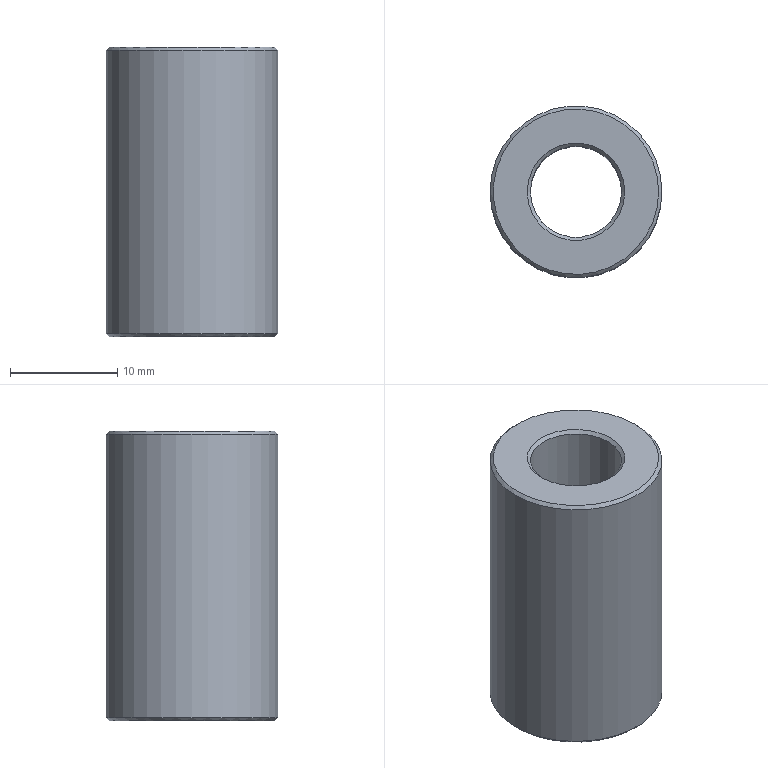Part | STEP file | 1 solid | 8 faces | box 16 x 16 x 27 mm | volume 3890 mm3 | cone 4 | cylinder 2 | plane 2 | commonest cylinder face diameters 8.5 x1 16 x1
STEP:
#1=CARTESIAN_POINT('',(0.,0.,0.));
#2=DIRECTION('',(0.,0.,1.));
#3=DIRECTION('',(1.,0.,0.));
#4=AXIS2_PLACEMENT_3D('',#1,#2,#3);
#5=CARTESIAN_POINT('',(1495.247,378.48,-53.681));
#6=VERTEX_POINT('',#5);
#7=CARTESIAN_POINT('',(1487.247,378.48,-53.681));
#8=DIRECTION('',(0.,0.,-1.));
#9=DIRECTION('',(1.,0.,0.));
#10=AXIS2_PLACEMENT_3D('',#7,#8,#9);
#11=CIRCLE('',#10,8.);
#12=CARTESIAN_POINT('',(1487.247,378.48,-53.381));
#13=DIRECTION('',(0.,0.,-1.));
#14=DIRECTION('',(-1.,0.,0.));
#15=AXIS2_PLACEMENT_3D('',#12,#13,#14);
#16=CYLINDRICAL_SURFACE('',#15,8.);
#17=CARTESIAN_POINT('',(3.142,0.3));
#18=DIRECTION('',(1.,0.));
#19=VECTOR('',#18,1.);
#20=LINE('',#17,#19);
#21=(GEOMETRIC_REPRESENTATION_CONTEXT(2)PARAMETRIC_REPRESENTATION_CONTEXT()REPRESENTATION_CONTEXT('',''));
#22=DEFINITIONAL_REPRESENTATION('',(#20),#21);
#23=PCURVE('',#16,#22);
#24=CARTESIAN_POINT('',(1487.247,378.48,-53.681));
#25=DIRECTION('',(0.,0.,-1.));
#26=DIRECTION('',(-1.,0.,0.));
#27=AXIS2_PLACEMENT_3D('',#24,#25,#26);
#28=CONICAL_SURFACE('',#27,8.,0.7854);
#29=CARTESIAN_POINT('',(3.142,0.));
#30=DIRECTION('',(1.,0.));
#31=VECTOR('',#30,1.);
#32=LINE('',#29,#31);
#33=(GEOMETRIC_REPRESENTATION_CONTEXT(2)PARAMETRIC_REPRESENTATION_CONTEXT()REPRESENTATION_CONTEXT('',''));
#34=DEFINITIONAL_REPRESENTATION('',(#32),#33);
#35=PCURVE('',#28,#34);
#36=SURFACE_CURVE('',#11,(#23,#35),.PCURVE_S1.);
#37=EDGE_CURVE('',#6,#6,#36,.T.);
#38=ORIENTED_EDGE('',*,*,#37,.T.);
#39=CARTESIAN_POINT('',(1495.247,378.48,-80.081));
#40=VERTEX_POINT('',#39);
#41=CARTESIAN_POINT('',(1495.247,378.48,-53.681));
#42=CARTESIAN_POINT('',(1495.247,378.48,-80.081));
#43=B_SPLINE_CURVE_WITH_KNOTS('',1,(#41,#42),.UNSPECIFIED.,.F.,.F.,(2,2),(0.3,26.7),.PIECEWISE_BEZIER_KNOTS.);
#44=CARTESIAN_POINT('',(9.425,0.));
#45=DIRECTION('',(0.,1.));
#46=VECTOR('',#45,1.);
#47=LINE('',#44,#46);
#48=(GEOMETRIC_REPRESENTATION_CONTEXT(2)PARAMETRIC_REPRESENTATION_CONTEXT()REPRESENTATION_CONTEXT('',''));
#49=DEFINITIONAL_REPRESENTATION('',(#47),#48);
#50=PCURVE('',#16,#49);
#51=CARTESIAN_POINT('',(3.142,0.));
#52=DIRECTION('',(0.,1.));
#53=VECTOR('',#52,1.);
#54=LINE('',#51,#53);
#55=(GEOMETRIC_REPRESENTATION_CONTEXT(2)PARAMETRIC_REPRESENTATION_CONTEXT()REPRESENTATION_CONTEXT('',''));
#56=DEFINITIONAL_REPRESENTATION('',(#54),#55);
#57=PCURVE('',#16,#56);
#58=SEAM_CURVE('',#43,(#50,#57),.PCURVE_S1.);
#59=EDGE_CURVE('',#6,#40,#58,.T.);
#60=ORIENTED_EDGE('',*,*,#59,.T.);
#61=CARTESIAN_POINT('',(1487.247,378.48,-80.081));
#62=DIRECTION('',(0.,0.,1.));
#63=DIRECTION('',(1.,0.,0.));
#64=AXIS2_PLACEMENT_3D('',#61,#62,#63);
#65=CIRCLE('',#64,8.);
#66=CARTESIAN_POINT('',(9.425,26.7));
#67=DIRECTION('',(-1.,0.));
#68=VECTOR('',#67,1.);
#69=LINE('',#66,#68);
#70=(GEOMETRIC_REPRESENTATION_CONTEXT(2)PARAMETRIC_REPRESENTATION_CONTEXT()REPRESENTATION_CONTEXT('',''));
#71=DEFINITIONAL_REPRESENTATION('',(#69),#70);
#72=PCURVE('',#16,#71);
#73=CARTESIAN_POINT('',(1487.247,378.48,-80.381));
#74=DIRECTION('',(0.,0.,1.));
#75=DIRECTION('',(1.,0.,0.));
#76=AXIS2_PLACEMENT_3D('',#73,#74,#75);
#77=CONICAL_SURFACE('',#76,7.7,0.7854);
#78=CARTESIAN_POINT('',(0.,0.3));
#79=DIRECTION('',(1.,0.));
#80=VECTOR('',#79,1.);
#81=LINE('',#78,#80);
#82=(GEOMETRIC_REPRESENTATION_CONTEXT(2)PARAMETRIC_REPRESENTATION_CONTEXT()REPRESENTATION_CONTEXT('',''));
#83=DEFINITIONAL_REPRESENTATION('',(#81),#82);
#84=PCURVE('',#77,#83);
#85=SURFACE_CURVE('',#65,(#72,#84),.PCURVE_S1.);
#86=EDGE_CURVE('',#40,#40,#85,.T.);
#87=ORIENTED_EDGE('',*,*,#86,.T.);
#88=ORIENTED_EDGE('',*,*,#59,.F.);
#89=EDGE_LOOP('',(#38,#60,#87,#88));
#90=FACE_BOUND('',#89,.T.);
#91=ADVANCED_FACE('',(#90),#16,.T.);
#92=CARTESIAN_POINT('',(1494.947,378.48,-53.381));
#93=VERTEX_POINT('',#92);
#94=CARTESIAN_POINT('',(1487.247,378.48,-53.381));
#95=DIRECTION('',(0.,0.,1.));
#96=DIRECTION('',(1.,0.,0.));
#97=AXIS2_PLACEMENT_3D('',#94,#95,#96);
#98=CIRCLE('',#97,7.7);
#99=CARTESIAN_POINT('',(1487.247,378.48,-53.381));
#100=DIRECTION('',(0.,0.,1.));
#101=DIRECTION('',(-1.,0.,0.));
#102=AXIS2_PLACEMENT_3D('',#99,#100,#101);
#103=PLANE('',#102);
#104=CARTESIAN_POINT('',(0.,0.));
#105=DIRECTION('',(-1.,0.));
#106=AXIS2_PLACEMENT_2D('',#104,#105);
#107=CIRCLE('',#106,7.7);
#108=(GEOMETRIC_REPRESENTATION_CONTEXT(2)PARAMETRIC_REPRESENTATION_CONTEXT()REPRESENTATION_CONTEXT('',''));
#109=DEFINITIONAL_REPRESENTATION('',(#107),#108);
#110=PCURVE('',#103,#109);
#111=CARTESIAN_POINT('',(9.425,-0.3));
#112=DIRECTION('',(-1.,0.));
#113=VECTOR('',#112,1.);
#114=LINE('',#111,#113);
#115=(GEOMETRIC_REPRESENTATION_CONTEXT(2)PARAMETRIC_REPRESENTATION_CONTEXT()REPRESENTATION_CONTEXT('',''));
#116=DEFINITIONAL_REPRESENTATION('',(#114),#115);
#117=PCURVE('',#28,#116);
#118=SURFACE_CURVE('',#98,(#110,#117),.PCURVE_S1.);
#119=EDGE_CURVE('',#93,#93,#118,.T.);
#120=ORIENTED_EDGE('',*,*,#119,.T.);
#121=EDGE_LOOP('',(#120));
#122=FACE_BOUND('',#121,.T.);
#123=CARTESIAN_POINT('',(1491.797,378.48,-53.381));
#124=VERTEX_POINT('',#123);
#125=CARTESIAN_POINT('',(1487.247,378.48,-53.381));
#126=DIRECTION('',(0.,0.,-1.));
#127=DIRECTION('',(1.,0.,0.));
#128=AXIS2_PLACEMENT_3D('',#125,#126,#127);
#129=CIRCLE('',#128,4.55);
#130=CARTESIAN_POINT('',(-4.55,0.));
#131=CARTESIAN_POINT('',(-4.55,7.881));
#132=CARTESIAN_POINT('',(2.275,3.94));
#133=CARTESIAN_POINT('',(9.1,0.));
#134=CARTESIAN_POINT('',(2.275,-3.94));
#135=CARTESIAN_POINT('',(-4.55,-7.881));
#136=CARTESIAN_POINT('',(-4.55,0.));
#137=(BOUNDED_CURVE()B_SPLINE_CURVE(2,(#130,#131,#132,#133,#134,#135,#136),.UNSPECIFIED.,.T.,.F.)B_SPLINE_CURVE_WITH_KNOTS((1,2,2,2,2,1),(-2.094,0.,2.094,4.189,6.283,8.378),.UNSPECIFIED.)CURVE()GEOMETRIC_REPRESENTATION_ITEM()RATIONAL_B_SPLINE_CURVE((1.,0.5,1.,0.5,1.,0.5,1.))REPRESENTATION_ITEM(''));
#138=(GEOMETRIC_REPRESENTATION_CONTEXT(2)PARAMETRIC_REPRESENTATION_CONTEXT()REPRESENTATION_CONTEXT('',''));
#139=DEFINITIONAL_REPRESENTATION('',(#137),#138);
#140=PCURVE('',#103,#139);
#141=CARTESIAN_POINT('',(1487.247,378.48,-53.681));
#142=DIRECTION('',(0.,0.,1.));
#143=DIRECTION('',(1.,0.,0.));
#144=AXIS2_PLACEMENT_3D('',#141,#142,#143);
#145=CONICAL_SURFACE('',#144,4.25,0.7854);
#146=CARTESIAN_POINT('',(6.283,0.3));
#147=DIRECTION('',(-1.,0.));
#148=VECTOR('',#147,1.);
#149=LINE('',#146,#148);
#150=(GEOMETRIC_REPRESENTATION_CONTEXT(2)PARAMETRIC_REPRESENTATION_CONTEXT()REPRESENTATION_CONTEXT('',''));
#151=DEFINITIONAL_REPRESENTATION('',(#149),#150);
#152=PCURVE('',#145,#151);
#153=SURFACE_CURVE('',#129,(#140,#152),.PCURVE_S1.);
#154=EDGE_CURVE('',#124,#124,#153,.T.);
#155=ORIENTED_EDGE('',*,*,#154,.T.);
#156=EDGE_LOOP('',(#155));
#157=FACE_BOUND('',#156,.T.);
#158=ADVANCED_FACE('',(#122,#157),#103,.T.);
#159=CARTESIAN_POINT('',(1491.497,378.48,-53.681));
#160=VERTEX_POINT('',#159);
#161=CARTESIAN_POINT('',(1487.247,378.48,-53.681));
#162=DIRECTION('',(0.,0.,1.));
#163=DIRECTION('',(1.,0.,0.));
#164=AXIS2_PLACEMENT_3D('',#161,#162,#163);
#165=CIRCLE('',#164,4.25);
#166=CARTESIAN_POINT('',(1487.247,378.48,-89.381));
#167=DIRECTION('',(0.,0.,1.));
#168=DIRECTION('',(-1.,0.,0.));
#169=AXIS2_PLACEMENT_3D('',#166,#167,#168);
#170=CYLINDRICAL_SURFACE('',#169,4.25);
#171=CARTESIAN_POINT('',(3.142,35.7));
#172=DIRECTION('',(1.,0.));
#173=VECTOR('',#172,1.);
#174=LINE('',#171,#173);
#175=(GEOMETRIC_REPRESENTATION_CONTEXT(2)PARAMETRIC_REPRESENTATION_CONTEXT()REPRESENTATION_CONTEXT('',''));
#176=DEFINITIONAL_REPRESENTATION('',(#174),#175);
#177=PCURVE('',#170,#176);
#178=CARTESIAN_POINT('',(0.,0.));
#179=DIRECTION('',(1.,0.));
#180=VECTOR('',#179,1.);
#181=LINE('',#178,#180);
#182=(GEOMETRIC_REPRESENTATION_CONTEXT(2)PARAMETRIC_REPRESENTATION_CONTEXT()REPRESENTATION_CONTEXT('',''));
#183=DEFINITIONAL_REPRESENTATION('',(#181),#182);
#184=PCURVE('',#145,#183);
#185=SURFACE_CURVE('',#165,(#177,#184),.PCURVE_S1.);
#186=EDGE_CURVE('',#160,#160,#185,.T.);
#187=ORIENTED_EDGE('',*,*,#186,.F.);
#188=CARTESIAN_POINT('',(1491.497,378.48,-80.081));
#189=VERTEX_POINT('',#188);
#190=CARTESIAN_POINT('',(1491.497,378.48,-80.081));
#191=CARTESIAN_POINT('',(1491.497,378.48,-53.681));
#192=B_SPLINE_CURVE_WITH_KNOTS('',1,(#190,#191),.UNSPECIFIED.,.F.,.F.,(2,2),(9.3,35.7),.PIECEWISE_BEZIER_KNOTS.);
#193=CARTESIAN_POINT('',(3.142,0.));
#194=DIRECTION('',(0.,1.));
#195=VECTOR('',#194,1.);
#196=LINE('',#193,#195);
#197=(GEOMETRIC_REPRESENTATION_CONTEXT(2)PARAMETRIC_REPRESENTATION_CONTEXT()REPRESENTATION_CONTEXT('',''));
#198=DEFINITIONAL_REPRESENTATION('',(#196),#197);
#199=PCURVE('',#170,#198);
#200=CARTESIAN_POINT('',(9.425,0.));
#201=DIRECTION('',(0.,1.));
#202=VECTOR('',#201,1.);
#203=LINE('',#200,#202);
#204=(GEOMETRIC_REPRESENTATION_CONTEXT(2)PARAMETRIC_REPRESENTATION_CONTEXT()REPRESENTATION_CONTEXT('',''));
#205=DEFINITIONAL_REPRESENTATION('',(#203),#204);
#206=PCURVE('',#170,#205);
#207=SEAM_CURVE('',#192,(#199,#206),.PCURVE_S1.);
#208=EDGE_CURVE('',#189,#160,#207,.T.);
#209=ORIENTED_EDGE('',*,*,#208,.F.);
#210=CARTESIAN_POINT('',(1487.247,378.48,-80.081));
#211=DIRECTION('',(0.,0.,-1.));
#212=DIRECTION('',(1.,0.,0.));
#213=AXIS2_PLACEMENT_3D('',#210,#211,#212);
#214=CIRCLE('',#213,4.25);
#215=CARTESIAN_POINT('',(9.425,9.3));
#216=DIRECTION('',(-1.,0.));
#217=VECTOR('',#216,1.);
#218=LINE('',#215,#217);
#219=(GEOMETRIC_REPRESENTATION_CONTEXT(2)PARAMETRIC_REPRESENTATION_CONTEXT()REPRESENTATION_CONTEXT('',''));
#220=DEFINITIONAL_REPRESENTATION('',(#218),#219);
#221=PCURVE('',#170,#220);
#222=CARTESIAN_POINT('',(1487.247,378.48,-80.081));
#223=DIRECTION('',(0.,0.,-1.));
#224=DIRECTION('',(-1.,0.,0.));
#225=AXIS2_PLACEMENT_3D('',#222,#223,#224);
#226=CONICAL_SURFACE('',#225,4.25,0.7854);
#227=CARTESIAN_POINT('',(3.142,0.));
#228=DIRECTION('',(1.,0.));
#229=VECTOR('',#228,1.);
#230=LINE('',#227,#229);
#231=(GEOMETRIC_REPRESENTATION_CONTEXT(2)PARAMETRIC_REPRESENTATION_CONTEXT()REPRESENTATION_CONTEXT('',''));
#232=DEFINITIONAL_REPRESENTATION('',(#230),#231);
#233=PCURVE('',#226,#232);
#234=SURFACE_CURVE('',#214,(#221,#233),.PCURVE_S1.);
#235=EDGE_CURVE('',#189,#189,#234,.T.);
#236=ORIENTED_EDGE('',*,*,#235,.F.);
#237=ORIENTED_EDGE('',*,*,#208,.T.);
#238=EDGE_LOOP('',(#187,#209,#236,#237));
#239=FACE_BOUND('',#238,.F.);
#240=ADVANCED_FACE('',(#239),#170,.F.);
#241=CARTESIAN_POINT('',(1494.947,378.48,-80.381));
#242=VERTEX_POINT('',#241);
#243=CARTESIAN_POINT('',(1487.247,378.48,-80.381));
#244=DIRECTION('',(0.,0.,-1.));
#245=DIRECTION('',(1.,0.,0.));
#246=AXIS2_PLACEMENT_3D('',#243,#244,#245);
#247=CIRCLE('',#246,7.7);
#248=CARTESIAN_POINT('',(1487.247,378.48,-80.381));
#249=DIRECTION('',(0.,0.,1.));
#250=DIRECTION('',(1.,0.,0.));
#251=AXIS2_PLACEMENT_3D('',#248,#249,#250);
#252=PLANE('',#251);
#253=CARTESIAN_POINT('',(7.7,0.));
#254=CARTESIAN_POINT('',(7.7,-13.337));
#255=CARTESIAN_POINT('',(-3.85,-6.668));
#256=CARTESIAN_POINT('',(-15.4,0.));
#257=CARTESIAN_POINT('',(-3.85,6.668));
#258=CARTESIAN_POINT('',(7.7,13.337));
#259=CARTESIAN_POINT('',(7.7,0.));
#260=(BOUNDED_CURVE()B_SPLINE_CURVE(2,(#253,#254,#255,#256,#257,#258,#259),.UNSPECIFIED.,.T.,.F.)B_SPLINE_CURVE_WITH_KNOTS((1,2,2,2,2,1),(-2.094,0.,2.094,4.189,6.283,8.378),.UNSPECIFIED.)CURVE()GEOMETRIC_REPRESENTATION_ITEM()RATIONAL_B_SPLINE_CURVE((1.,0.5,1.,0.5,1.,0.5,1.))REPRESENTATION_ITEM(''));
#261=(GEOMETRIC_REPRESENTATION_CONTEXT(2)PARAMETRIC_REPRESENTATION_CONTEXT()REPRESENTATION_CONTEXT('',''));
#262=DEFINITIONAL_REPRESENTATION('',(#260),#261);
#263=PCURVE('',#252,#262);
#264=CARTESIAN_POINT('',(6.283,0.));
#265=DIRECTION('',(-1.,0.));
#266=VECTOR('',#265,1.);
#267=LINE('',#264,#266);
#268=(GEOMETRIC_REPRESENTATION_CONTEXT(2)PARAMETRIC_REPRESENTATION_CONTEXT()REPRESENTATION_CONTEXT('',''));
#269=DEFINITIONAL_REPRESENTATION('',(#267),#268);
#270=PCURVE('',#77,#269);
#271=SURFACE_CURVE('',#247,(#263,#270),.PCURVE_S1.);
#272=EDGE_CURVE('',#242,#242,#271,.T.);
#273=ORIENTED_EDGE('',*,*,#272,.T.);
#274=EDGE_LOOP('',(#273));
#275=FACE_BOUND('',#274,.T.);
#276=CARTESIAN_POINT('',(1491.797,378.48,-80.381));
#277=VERTEX_POINT('',#276);
#278=CARTESIAN_POINT('',(1487.247,378.48,-80.381));
#279=DIRECTION('',(0.,0.,1.));
#280=DIRECTION('',(1.,0.,0.));
#281=AXIS2_PLACEMENT_3D('',#278,#279,#280);
#282=CIRCLE('',#281,4.55);
#283=CARTESIAN_POINT('',(0.,0.));
#284=DIRECTION('',(1.,0.));
#285=AXIS2_PLACEMENT_2D('',#283,#284);
#286=CIRCLE('',#285,4.55);
#287=(GEOMETRIC_REPRESENTATION_CONTEXT(2)PARAMETRIC_REPRESENTATION_CONTEXT()REPRESENTATION_CONTEXT('',''));
#288=DEFINITIONAL_REPRESENTATION('',(#286),#287);
#289=PCURVE('',#252,#288);
#290=CARTESIAN_POINT('',(9.425,0.3));
#291=DIRECTION('',(-1.,0.));
#292=VECTOR('',#291,1.);
#293=LINE('',#290,#292);
#294=(GEOMETRIC_REPRESENTATION_CONTEXT(2)PARAMETRIC_REPRESENTATION_CONTEXT()REPRESENTATION_CONTEXT('',''));
#295=DEFINITIONAL_REPRESENTATION('',(#293),#294);
#296=PCURVE('',#226,#295);
#297=SURFACE_CURVE('',#282,(#289,#296),.PCURVE_S1.);
#298=EDGE_CURVE('',#277,#277,#297,.T.);
#299=ORIENTED_EDGE('',*,*,#298,.T.);
#300=EDGE_LOOP('',(#299));
#301=FACE_BOUND('',#300,.T.);
#302=ADVANCED_FACE('',(#275,#301),#252,.F.);
#303=ORIENTED_EDGE('',*,*,#86,.F.);
#304=CARTESIAN_POINT('',(1494.947,378.48,-80.381));
#305=CARTESIAN_POINT('',(1495.247,378.48,-80.081));
#306=B_SPLINE_CURVE_WITH_KNOTS('',1,(#304,#305),.UNSPECIFIED.,.F.,.F.,(2,2),(0.,0.4243),.PIECEWISE_BEZIER_KNOTS.);
#307=CARTESIAN_POINT('',(0.,0.));
#308=DIRECTION('',(0.,1.));
#309=VECTOR('',#308,1.);
#310=LINE('',#307,#309);
#311=(GEOMETRIC_REPRESENTATION_CONTEXT(2)PARAMETRIC_REPRESENTATION_CONTEXT()REPRESENTATION_CONTEXT('',''));
#312=DEFINITIONAL_REPRESENTATION('',(#310),#311);
#313=PCURVE('',#77,#312);
#314=CARTESIAN_POINT('',(6.283,0.));
#315=DIRECTION('',(0.,1.));
#316=VECTOR('',#315,1.);
#317=LINE('',#314,#316);
#318=(GEOMETRIC_REPRESENTATION_CONTEXT(2)PARAMETRIC_REPRESENTATION_CONTEXT()REPRESENTATION_CONTEXT('',''));
#319=DEFINITIONAL_REPRESENTATION('',(#317),#318);
#320=PCURVE('',#77,#319);
#321=SEAM_CURVE('',#306,(#313,#320),.PCURVE_S1.);
#322=EDGE_CURVE('',#242,#40,#321,.T.);
#323=ORIENTED_EDGE('',*,*,#322,.F.);
#324=ORIENTED_EDGE('',*,*,#272,.F.);
#325=ORIENTED_EDGE('',*,*,#322,.T.);
#326=EDGE_LOOP('',(#303,#323,#324,#325));
#327=FACE_BOUND('',#326,.T.);
#328=ADVANCED_FACE('',(#327),#77,.T.);
#329=ORIENTED_EDGE('',*,*,#298,.T.);
#330=CARTESIAN_POINT('',(1491.497,378.48,-80.081));
#331=CARTESIAN_POINT('',(1491.797,378.48,-80.381));
#332=B_SPLINE_CURVE_WITH_KNOTS('',1,(#330,#331),.UNSPECIFIED.,.F.,.F.,(2,2),(0.,0.4243),.PIECEWISE_BEZIER_KNOTS.);
#333=CARTESIAN_POINT('',(3.142,0.));
#334=DIRECTION('',(0.,1.));
#335=VECTOR('',#334,1.);
#336=LINE('',#333,#335);
#337=(GEOMETRIC_REPRESENTATION_CONTEXT(2)PARAMETRIC_REPRESENTATION_CONTEXT()REPRESENTATION_CONTEXT('',''));
#338=DEFINITIONAL_REPRESENTATION('',(#336),#337);
#339=PCURVE('',#226,#338);
#340=CARTESIAN_POINT('',(9.425,0.));
#341=DIRECTION('',(0.,1.));
#342=VECTOR('',#341,1.);
#343=LINE('',#340,#342);
#344=(GEOMETRIC_REPRESENTATION_CONTEXT(2)PARAMETRIC_REPRESENTATION_CONTEXT()REPRESENTATION_CONTEXT('',''));
#345=DEFINITIONAL_REPRESENTATION('',(#343),#344);
#346=PCURVE('',#226,#345);
#347=SEAM_CURVE('',#332,(#339,#346),.PCURVE_S1.);
#348=EDGE_CURVE('',#189,#277,#347,.T.);
#349=ORIENTED_EDGE('',*,*,#348,.F.);
#350=ORIENTED_EDGE('',*,*,#235,.T.);
#351=ORIENTED_EDGE('',*,*,#348,.T.);
#352=EDGE_LOOP('',(#329,#349,#350,#351));
#353=FACE_BOUND('',#352,.F.);
#354=ADVANCED_FACE('',(#353),#226,.F.);
#355=ORIENTED_EDGE('',*,*,#154,.T.);
#356=CARTESIAN_POINT('',(1491.497,378.48,-53.681));
#357=CARTESIAN_POINT('',(1491.797,378.48,-53.381));
#358=B_SPLINE_CURVE_WITH_KNOTS('',1,(#356,#357),.UNSPECIFIED.,.F.,.F.,(2,2),(0.,0.4243),.PIECEWISE_BEZIER_KNOTS.);
#359=CARTESIAN_POINT('',(0.,0.));
#360=DIRECTION('',(0.,1.));
#361=VECTOR('',#360,1.);
#362=LINE('',#359,#361);
#363=(GEOMETRIC_REPRESENTATION_CONTEXT(2)PARAMETRIC_REPRESENTATION_CONTEXT()REPRESENTATION_CONTEXT('',''));
#364=DEFINITIONAL_REPRESENTATION('',(#362),#363);
#365=PCURVE('',#145,#364);
#366=CARTESIAN_POINT('',(6.283,0.));
#367=DIRECTION('',(0.,1.));
#368=VECTOR('',#367,1.);
#369=LINE('',#366,#368);
#370=(GEOMETRIC_REPRESENTATION_CONTEXT(2)PARAMETRIC_REPRESENTATION_CONTEXT()REPRESENTATION_CONTEXT('',''));
#371=DEFINITIONAL_REPRESENTATION('',(#369),#370);
#372=PCURVE('',#145,#371);
#373=SEAM_CURVE('',#358,(#365,#372),.PCURVE_S1.);
#374=EDGE_CURVE('',#160,#124,#373,.T.);
#375=ORIENTED_EDGE('',*,*,#374,.F.);
#376=ORIENTED_EDGE('',*,*,#186,.T.);
#377=ORIENTED_EDGE('',*,*,#374,.T.);
#378=EDGE_LOOP('',(#355,#375,#376,#377));
#379=FACE_BOUND('',#378,.F.);
#380=ADVANCED_FACE('',(#379),#145,.F.);
#381=ORIENTED_EDGE('',*,*,#119,.F.);
#382=CARTESIAN_POINT('',(1494.947,378.48,-53.381));
#383=CARTESIAN_POINT('',(1495.247,378.48,-53.681));
#384=B_SPLINE_CURVE_WITH_KNOTS('',1,(#382,#383),.UNSPECIFIED.,.F.,.F.,(2,2),(-0.4243,0.),.PIECEWISE_BEZIER_KNOTS.);
#385=CARTESIAN_POINT('',(9.425,0.));
#386=DIRECTION('',(0.,1.));
#387=VECTOR('',#386,1.);
#388=LINE('',#385,#387);
#389=(GEOMETRIC_REPRESENTATION_CONTEXT(2)PARAMETRIC_REPRESENTATION_CONTEXT()REPRESENTATION_CONTEXT('',''));
#390=DEFINITIONAL_REPRESENTATION('',(#388),#389);
#391=PCURVE('',#28,#390);
#392=CARTESIAN_POINT('',(3.142,0.));
#393=DIRECTION('',(0.,1.));
#394=VECTOR('',#393,1.);
#395=LINE('',#392,#394);
#396=(GEOMETRIC_REPRESENTATION_CONTEXT(2)PARAMETRIC_REPRESENTATION_CONTEXT()REPRESENTATION_CONTEXT('',''));
#397=DEFINITIONAL_REPRESENTATION('',(#395),#396);
#398=PCURVE('',#28,#397);
#399=SEAM_CURVE('',#384,(#391,#398),.PCURVE_S1.);
#400=EDGE_CURVE('',#93,#6,#399,.T.);
#401=ORIENTED_EDGE('',*,*,#400,.T.);
#402=ORIENTED_EDGE('',*,*,#37,.F.);
#403=ORIENTED_EDGE('',*,*,#400,.F.);
#404=EDGE_LOOP('',(#381,#401,#402,#403));
#405=FACE_BOUND('',#404,.T.);
#406=ADVANCED_FACE('',(#405),#28,.T.);
#407=CLOSED_SHELL('',(#91,#158,#240,#302,#328,#354,#380,#406));
#408=MANIFOLD_SOLID_BREP('',#407);
#409=(LENGTH_UNIT()NAMED_UNIT(*)SI_UNIT(.MILLI.,.METRE.));
#410=UNCERTAINTY_MEASURE_WITH_UNIT(LENGTH_MEASURE(0.00001),#409,'','');
#411=(NAMED_UNIT(*)PLANE_ANGLE_UNIT()SI_UNIT($,.RADIAN.));
#412=(NAMED_UNIT(*)SI_UNIT($,.STERADIAN.)SOLID_ANGLE_UNIT());
#413=(GEOMETRIC_REPRESENTATION_CONTEXT(3)GLOBAL_UNCERTAINTY_ASSIGNED_CONTEXT((#410))GLOBAL_UNIT_ASSIGNED_CONTEXT((#409,#411,#412))REPRESENTATION_CONTEXT('',''));
#414=ADVANCED_BREP_SHAPE_REPRESENTATION('',(#4,#408),#413);